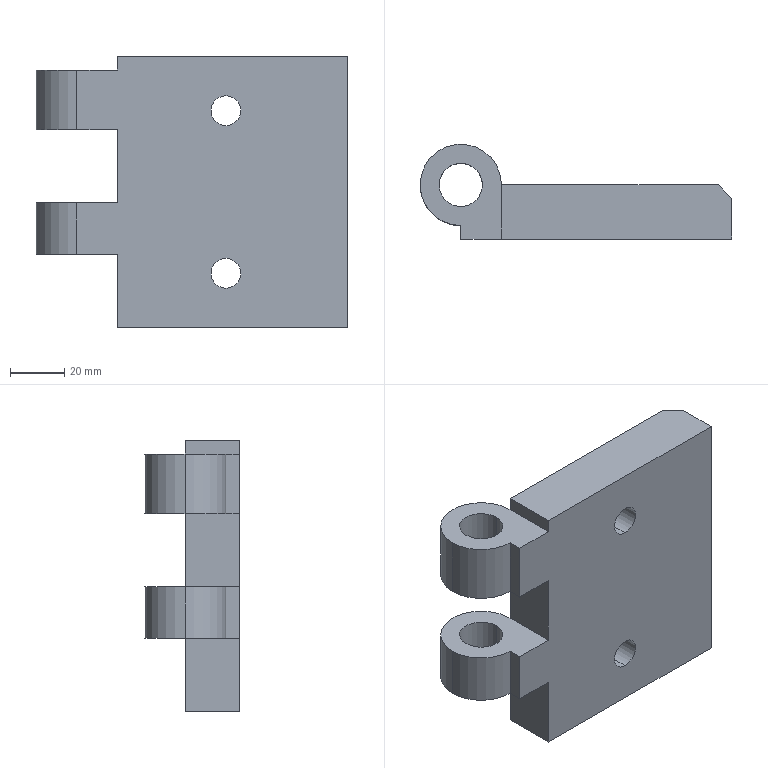Part | SolidWorks | features ICE 2, 3DProfileFeature 1, Chamfer 1, Extrusion 1, HoleWzd 1, MirrorPattern 1 | 1 solid | 33 faces | box 115 x 35 x 100 mm | volume 190454 mm3 | plane 17 | cylinder 16 | commonest cylinder face diameters 11 x4 16 x4 22 x4 30 x4
STEP:
#1=CARTESIAN_POINT('',(5.,9.5,19.));
#2=VERTEX_POINT('',#1);
#3=CARTESIAN_POINT('',(5.,9.5,41.));
#4=VERTEX_POINT('',#3);
#5=CARTESIAN_POINT('',(5.,9.5,30.));
#6=DIRECTION('',(0.,1.,0.));
#7=DIRECTION('',(0.,0.,1.));
#8=AXIS2_PLACEMENT_3D('',#5,#6,#7);
#9=CIRCLE('',#8,11.);
#10=EDGE_CURVE('',#2,#4,#9,.T.);
#11=ORIENTED_EDGE('',*,*,#10,.F.);
#12=CARTESIAN_POINT('',(5.,10.,19.));
#13=VERTEX_POINT('',#12);
#14=CARTESIAN_POINT('',(5.,10.,19.));
#15=DIRECTION('',(0.,1.,0.));
#16=VECTOR('',#15,1000.);
#17=LINE('',#14,#16);
#18=EDGE_CURVE('',#2,#13,#17,.T.);
#19=ORIENTED_EDGE('',*,*,#18,.T.);
#20=CARTESIAN_POINT('',(5.,10.,41.));
#21=VERTEX_POINT('',#20);
#22=CARTESIAN_POINT('',(5.,10.,30.));
#23=DIRECTION('',(0.,1.,0.));
#24=DIRECTION('',(0.,0.,1.));
#25=AXIS2_PLACEMENT_3D('',#22,#23,#24);
#26=CIRCLE('',#25,11.);
#27=EDGE_CURVE('',#13,#21,#26,.T.);
#28=ORIENTED_EDGE('',*,*,#27,.T.);
#29=CARTESIAN_POINT('',(5.,10.,41.));
#30=DIRECTION('',(0.,1.,0.));
#31=VECTOR('',#30,1000.);
#32=LINE('',#29,#31);
#33=EDGE_CURVE('',#4,#21,#32,.T.);
#34=ORIENTED_EDGE('',*,*,#33,.F.);
#35=EDGE_LOOP('',(#11,#19,#28,#34));
#36=FACE_OUTER_BOUND('',#35,.T.);
#37=CARTESIAN_POINT('',(5.,10.,30.));
#38=DIRECTION('',(0.,1.,0.));
#39=DIRECTION('',(0.,0.,1.));
#40=AXIS2_PLACEMENT_3D('',#37,#38,#39);
#41=CYLINDRICAL_SURFACE('',#40,11.);
#42=ADVANCED_FACE('',(#36),#41,.F.);
#43=CARTESIAN_POINT('',(5.,-10.,24.5));
#44=VERTEX_POINT('',#43);
#45=CARTESIAN_POINT('',(5.,-10.,35.5));
#46=VERTEX_POINT('',#45);
#47=CARTESIAN_POINT('',(5.,-10.,30.));
#48=DIRECTION('',(0.,1.,0.));
#49=DIRECTION('',(0.,0.,1.));
#50=AXIS2_PLACEMENT_3D('',#47,#48,#49);
#51=CIRCLE('',#50,5.5);
#52=EDGE_CURVE('',#44,#46,#51,.T.);
#53=ORIENTED_EDGE('',*,*,#52,.F.);
#54=CARTESIAN_POINT('',(5.,9.5,24.5));
#55=VERTEX_POINT('',#54);
#56=CARTESIAN_POINT('',(5.,10.,24.5));
#57=DIRECTION('',(0.,1.,0.));
#58=VECTOR('',#57,1000.);
#59=LINE('',#56,#58);
#60=EDGE_CURVE('',#44,#55,#59,.T.);
#61=ORIENTED_EDGE('',*,*,#60,.T.);
#62=CARTESIAN_POINT('',(5.,9.5,35.5));
#63=VERTEX_POINT('',#62);
#64=CARTESIAN_POINT('',(5.,9.5,30.));
#65=DIRECTION('',(0.,1.,0.));
#66=DIRECTION('',(0.,0.,1.));
#67=AXIS2_PLACEMENT_3D('',#64,#65,#66);
#68=CIRCLE('',#67,5.5);
#69=EDGE_CURVE('',#55,#63,#68,.T.);
#70=ORIENTED_EDGE('',*,*,#69,.T.);
#71=CARTESIAN_POINT('',(5.,10.,35.5));
#72=DIRECTION('',(0.,1.,0.));
#73=VECTOR('',#72,1000.);
#74=LINE('',#71,#73);
#75=EDGE_CURVE('',#46,#63,#74,.T.);
#76=ORIENTED_EDGE('',*,*,#75,.F.);
#77=EDGE_LOOP('',(#53,#61,#70,#76));
#78=FACE_OUTER_BOUND('',#77,.T.);
#79=CARTESIAN_POINT('',(5.,10.,30.));
#80=DIRECTION('',(0.,1.,0.));
#81=DIRECTION('',(0.,0.,1.));
#82=AXIS2_PLACEMENT_3D('',#79,#80,#81);
#83=CYLINDRICAL_SURFACE('',#82,5.5);
#84=ADVANCED_FACE('',(#78),#83,.F.);
#85=CARTESIAN_POINT('',(5.,9.5,-41.));
#86=VERTEX_POINT('',#85);
#87=CARTESIAN_POINT('',(5.,9.5,-19.));
#88=VERTEX_POINT('',#87);
#89=CARTESIAN_POINT('',(5.,9.5,-30.));
#90=DIRECTION('',(0.,1.,0.));
#91=DIRECTION('',(0.,0.,1.));
#92=AXIS2_PLACEMENT_3D('',#89,#90,#91);
#93=CIRCLE('',#92,11.);
#94=EDGE_CURVE('',#86,#88,#93,.T.);
#95=ORIENTED_EDGE('',*,*,#94,.F.);
#96=CARTESIAN_POINT('',(5.,10.,-41.));
#97=VERTEX_POINT('',#96);
#98=CARTESIAN_POINT('',(5.,10.,-41.));
#99=DIRECTION('',(0.,1.,0.));
#100=VECTOR('',#99,1000.);
#101=LINE('',#98,#100);
#102=EDGE_CURVE('',#86,#97,#101,.T.);
#103=ORIENTED_EDGE('',*,*,#102,.T.);
#104=CARTESIAN_POINT('',(5.,10.,-19.));
#105=VERTEX_POINT('',#104);
#106=CARTESIAN_POINT('',(5.,10.,-30.));
#107=DIRECTION('',(0.,1.,0.));
#108=DIRECTION('',(0.,0.,1.));
#109=AXIS2_PLACEMENT_3D('',#106,#107,#108);
#110=CIRCLE('',#109,11.);
#111=EDGE_CURVE('',#97,#105,#110,.T.);
#112=ORIENTED_EDGE('',*,*,#111,.T.);
#113=CARTESIAN_POINT('',(5.,10.,-19.));
#114=DIRECTION('',(0.,1.,0.));
#115=VECTOR('',#114,1000.);
#116=LINE('',#113,#115);
#117=EDGE_CURVE('',#88,#105,#116,.T.);
#118=ORIENTED_EDGE('',*,*,#117,.F.);
#119=EDGE_LOOP('',(#95,#103,#112,#118));
#120=FACE_OUTER_BOUND('',#119,.T.);
#121=CARTESIAN_POINT('',(5.,10.,-30.));
#122=DIRECTION('',(0.,1.,0.));
#123=DIRECTION('',(0.,0.,1.));
#124=AXIS2_PLACEMENT_3D('',#121,#122,#123);
#125=CYLINDRICAL_SURFACE('',#124,11.);
#126=ADVANCED_FACE('',(#120),#125,.F.);
#127=CARTESIAN_POINT('',(5.,-10.,-35.5));
#128=VERTEX_POINT('',#127);
#129=CARTESIAN_POINT('',(5.,-10.,-24.5));
#130=VERTEX_POINT('',#129);
#131=CARTESIAN_POINT('',(5.,-10.,-30.));
#132=DIRECTION('',(0.,1.,0.));
#133=DIRECTION('',(0.,0.,1.));
#134=AXIS2_PLACEMENT_3D('',#131,#132,#133);
#135=CIRCLE('',#134,5.5);
#136=EDGE_CURVE('',#128,#130,#135,.T.);
#137=ORIENTED_EDGE('',*,*,#136,.F.);
#138=CARTESIAN_POINT('',(5.,9.5,-35.5));
#139=VERTEX_POINT('',#138);
#140=CARTESIAN_POINT('',(5.,10.,-35.5));
#141=DIRECTION('',(0.,1.,0.));
#142=VECTOR('',#141,1000.);
#143=LINE('',#140,#142);
#144=EDGE_CURVE('',#128,#139,#143,.T.);
#145=ORIENTED_EDGE('',*,*,#144,.T.);
#146=CARTESIAN_POINT('',(5.,9.5,-24.5));
#147=VERTEX_POINT('',#146);
#148=CARTESIAN_POINT('',(5.,9.5,-30.));
#149=DIRECTION('',(0.,1.,0.));
#150=DIRECTION('',(0.,0.,1.));
#151=AXIS2_PLACEMENT_3D('',#148,#149,#150);
#152=CIRCLE('',#151,5.5);
#153=EDGE_CURVE('',#139,#147,#152,.T.);
#154=ORIENTED_EDGE('',*,*,#153,.T.);
#155=CARTESIAN_POINT('',(5.,10.,-24.5));
#156=DIRECTION('',(0.,1.,0.));
#157=VECTOR('',#156,1000.);
#158=LINE('',#155,#157);
#159=EDGE_CURVE('',#130,#147,#158,.T.);
#160=ORIENTED_EDGE('',*,*,#159,.F.);
#161=EDGE_LOOP('',(#137,#145,#154,#160));
#162=FACE_OUTER_BOUND('',#161,.T.);
#163=CARTESIAN_POINT('',(5.,10.,-30.));
#164=DIRECTION('',(0.,1.,0.));
#165=DIRECTION('',(0.,0.,1.));
#166=AXIS2_PLACEMENT_3D('',#163,#164,#165);
#167=CYLINDRICAL_SURFACE('',#166,5.5);
#168=ADVANCED_FACE('',(#162),#167,.F.);
#169=CARTESIAN_POINT('',(-42.,10.,-22.997));
#170=VERTEX_POINT('',#169);
#171=CARTESIAN_POINT('',(-58.,10.,-22.997));
#172=VERTEX_POINT('',#171);
#173=CARTESIAN_POINT('',(-50.,10.,-22.997));
#174=DIRECTION('',(0.,0.,-1.));
#175=DIRECTION('',(1.,0.,0.));
#176=AXIS2_PLACEMENT_3D('',#173,#174,#175);
#177=CIRCLE('',#176,8.);
#178=EDGE_CURVE('',#170,#172,#177,.T.);
#179=ORIENTED_EDGE('',*,*,#178,.T.);
#180=CARTESIAN_POINT('',(-58.,10.,-3.997));
#181=VERTEX_POINT('',#180);
#182=CARTESIAN_POINT('',(-58.,10.,-50.));
#183=DIRECTION('',(0.,0.,1.));
#184=VECTOR('',#183,1000.);
#185=LINE('',#182,#184);
#186=EDGE_CURVE('',#172,#181,#185,.T.);
#187=ORIENTED_EDGE('',*,*,#186,.T.);
#188=CARTESIAN_POINT('',(-42.,10.,-3.997));
#189=VERTEX_POINT('',#188);
#190=CARTESIAN_POINT('',(-50.,10.,-3.997));
#191=DIRECTION('',(0.,0.,-1.));
#192=DIRECTION('',(1.,0.,0.));
#193=AXIS2_PLACEMENT_3D('',#190,#191,#192);
#194=CIRCLE('',#193,8.);
#195=EDGE_CURVE('',#189,#181,#194,.T.);
#196=ORIENTED_EDGE('',*,*,#195,.F.);
#197=CARTESIAN_POINT('',(-42.,10.,-50.));
#198=DIRECTION('',(0.,0.,1.));
#199=VECTOR('',#198,1000.);
#200=LINE('',#197,#199);
#201=EDGE_CURVE('',#170,#189,#200,.T.);
#202=ORIENTED_EDGE('',*,*,#201,.F.);
#203=EDGE_LOOP('',(#179,#187,#196,#202));
#204=FACE_OUTER_BOUND('',#203,.T.);
#205=CARTESIAN_POINT('',(-50.,10.,-50.));
#206=DIRECTION('',(0.,0.,1.));
#207=DIRECTION('',(1.,0.,0.));
#208=AXIS2_PLACEMENT_3D('',#205,#206,#207);
#209=CYLINDRICAL_SURFACE('',#208,8.);
#210=ADVANCED_FACE('',(#204),#209,.F.);
#211=CARTESIAN_POINT('',(-42.,10.,23.003));
#212=VERTEX_POINT('',#211);
#213=CARTESIAN_POINT('',(-58.,10.,23.003));
#214=VERTEX_POINT('',#213);
#215=CARTESIAN_POINT('',(-50.,10.,23.003));
#216=DIRECTION('',(0.,0.,-1.));
#217=DIRECTION('',(1.,0.,0.));
#218=AXIS2_PLACEMENT_3D('',#215,#216,#217);
#219=CIRCLE('',#218,8.);
#220=EDGE_CURVE('',#212,#214,#219,.T.);
#221=ORIENTED_EDGE('',*,*,#220,.T.);
#222=CARTESIAN_POINT('',(-58.,10.,45.));
#223=VERTEX_POINT('',#222);
#224=CARTESIAN_POINT('',(-58.,10.,-50.));
#225=DIRECTION('',(0.,0.,1.));
#226=VECTOR('',#225,1000.);
#227=LINE('',#224,#226);
#228=EDGE_CURVE('',#214,#223,#227,.T.);
#229=ORIENTED_EDGE('',*,*,#228,.T.);
#230=CARTESIAN_POINT('',(-42.,10.,45.));
#231=VERTEX_POINT('',#230);
#232=CARTESIAN_POINT('',(-50.,10.,45.));
#233=DIRECTION('',(0.,0.,1.));
#234=DIRECTION('',(-1.,0.,0.));
#235=AXIS2_PLACEMENT_3D('',#232,#233,#234);
#236=CIRCLE('',#235,8.);
#237=EDGE_CURVE('',#223,#231,#236,.T.);
#238=ORIENTED_EDGE('',*,*,#237,.T.);
#239=CARTESIAN_POINT('',(-42.,10.,-50.));
#240=DIRECTION('',(0.,0.,1.));
#241=VECTOR('',#240,1000.);
#242=LINE('',#239,#241);
#243=EDGE_CURVE('',#212,#231,#242,.T.);
#244=ORIENTED_EDGE('',*,*,#243,.F.);
#245=EDGE_LOOP('',(#221,#229,#238,#244));
#246=FACE_OUTER_BOUND('',#245,.T.);
#247=CARTESIAN_POINT('',(-50.,10.,-50.));
#248=DIRECTION('',(0.,0.,1.));
#249=DIRECTION('',(1.,0.,0.));
#250=AXIS2_PLACEMENT_3D('',#247,#248,#249);
#251=CYLINDRICAL_SURFACE('',#250,8.);
#252=ADVANCED_FACE('',(#246),#251,.F.);
#253=CARTESIAN_POINT('',(-50.,-5.,45.));
#254=VERTEX_POINT('',#253);
#255=CARTESIAN_POINT('',(-65.,10.,45.));
#256=VERTEX_POINT('',#255);
#257=CARTESIAN_POINT('',(-50.,10.,45.));
#258=DIRECTION('',(0.,0.,-1.));
#259=DIRECTION('',(-1.,0.,0.));
#260=AXIS2_PLACEMENT_3D('',#257,#258,#259);
#261=CIRCLE('',#260,15.);
#262=EDGE_CURVE('',#254,#256,#261,.T.);
#263=ORIENTED_EDGE('',*,*,#262,.T.);
#264=CARTESIAN_POINT('',(-65.,10.,23.003));
#265=VERTEX_POINT('',#264);
#266=CARTESIAN_POINT('',(-65.,10.,50.));
#267=DIRECTION('',(0.,0.,-1.));
#268=VECTOR('',#267,1000.);
#269=LINE('',#266,#268);
#270=EDGE_CURVE('',#256,#265,#269,.T.);
#271=ORIENTED_EDGE('',*,*,#270,.T.);
#272=CARTESIAN_POINT('',(-50.,-5.,23.003));
#273=VERTEX_POINT('',#272);
#274=CARTESIAN_POINT('',(-50.,10.,23.003));
#275=DIRECTION('',(0.,0.,1.));
#276=DIRECTION('',(1.,0.,0.));
#277=AXIS2_PLACEMENT_3D('',#274,#275,#276);
#278=CIRCLE('',#277,15.);
#279=EDGE_CURVE('',#265,#273,#278,.T.);
#280=ORIENTED_EDGE('',*,*,#279,.T.);
#281=CARTESIAN_POINT('',(-50.,-5.,50.));
#282=DIRECTION('',(0.,0.,-1.));
#283=VECTOR('',#282,1000.);
#284=LINE('',#281,#283);
#285=EDGE_CURVE('',#254,#273,#284,.T.);
#286=ORIENTED_EDGE('',*,*,#285,.F.);
#287=EDGE_LOOP('',(#263,#271,#280,#286));
#288=FACE_OUTER_BOUND('',#287,.T.);
#289=CARTESIAN_POINT('',(-50.,10.,50.));
#290=DIRECTION('',(0.,0.,-1.));
#291=DIRECTION('',(-1.,0.,0.));
#292=AXIS2_PLACEMENT_3D('',#289,#290,#291);
#293=CYLINDRICAL_SURFACE('',#292,15.);
#294=ADVANCED_FACE('',(#288),#293,.T.);
#295=CARTESIAN_POINT('',(-65.,10.,-3.997));
#296=VERTEX_POINT('',#295);
#297=CARTESIAN_POINT('',(-50.,-5.,-3.997));
#298=VERTEX_POINT('',#297);
#299=CARTESIAN_POINT('',(-50.,10.,-3.997));
#300=DIRECTION('',(0.,0.,1.));
#301=DIRECTION('',(1.,0.,0.));
#302=AXIS2_PLACEMENT_3D('',#299,#300,#301);
#303=CIRCLE('',#302,15.);
#304=EDGE_CURVE('',#296,#298,#303,.T.);
#305=ORIENTED_EDGE('',*,*,#304,.F.);
#306=CARTESIAN_POINT('',(-65.,10.,-22.997));
#307=VERTEX_POINT('',#306);
#308=CARTESIAN_POINT('',(-65.,10.,50.));
#309=DIRECTION('',(0.,0.,-1.));
#310=VECTOR('',#309,1000.);
#311=LINE('',#308,#310);
#312=EDGE_CURVE('',#296,#307,#311,.T.);
#313=ORIENTED_EDGE('',*,*,#312,.T.);
#314=CARTESIAN_POINT('',(-50.,-5.,-22.997));
#315=VERTEX_POINT('',#314);
#316=CARTESIAN_POINT('',(-50.,10.,-22.997));
#317=DIRECTION('',(0.,0.,1.));
#318=DIRECTION('',(1.,0.,0.));
#319=AXIS2_PLACEMENT_3D('',#316,#317,#318);
#320=CIRCLE('',#319,15.);
#321=EDGE_CURVE('',#307,#315,#320,.T.);
#322=ORIENTED_EDGE('',*,*,#321,.T.);
#323=CARTESIAN_POINT('',(-50.,-5.,50.));
#324=DIRECTION('',(0.,0.,-1.));
#325=VECTOR('',#324,1000.);
#326=LINE('',#323,#325);
#327=EDGE_CURVE('',#298,#315,#326,.T.);
#328=ORIENTED_EDGE('',*,*,#327,.F.);
#329=EDGE_LOOP('',(#305,#313,#322,#328));
#330=FACE_OUTER_BOUND('',#329,.T.);
#331=CARTESIAN_POINT('',(-50.,10.,50.));
#332=DIRECTION('',(0.,0.,-1.));
#333=DIRECTION('',(-1.,0.,0.));
#334=AXIS2_PLACEMENT_3D('',#331,#332,#333);
#335=CYLINDRICAL_SURFACE('',#334,15.);
#336=ADVANCED_FACE('',(#330),#335,.T.);
#337=CARTESIAN_POINT('',(5.,10.,30.));
#338=DIRECTION('',(0.,1.,0.));
#339=DIRECTION('',(0.,0.,1.));
#340=AXIS2_PLACEMENT_3D('',#337,#338,#339);
#341=CIRCLE('',#340,11.);
#342=EDGE_CURVE('',#21,#13,#341,.T.);
#343=ORIENTED_EDGE('',*,*,#342,.F.);
#344=ORIENTED_EDGE('',*,*,#27,.F.);
#345=EDGE_LOOP('',(#343,#344));
#346=FACE_BOUND('',#345,.T.);
#347=CARTESIAN_POINT('',(45.,10.,50.));
#348=VERTEX_POINT('',#347);
#349=CARTESIAN_POINT('',(-35.,10.,50.));
#350=VERTEX_POINT('',#349);
#351=CARTESIAN_POINT('',(-35.,10.,50.));
#352=DIRECTION('',(-1.,0.,0.));
#353=VECTOR('',#352,1000.);
#354=LINE('',#351,#353);
#355=EDGE_CURVE('',#348,#350,#354,.T.);
#356=ORIENTED_EDGE('',*,*,#355,.F.);
#357=CARTESIAN_POINT('',(45.,10.,-50.));
#358=VERTEX_POINT('',#357);
#359=CARTESIAN_POINT('',(45.,10.,50.));
#360=DIRECTION('',(0.,0.,-1.));
#361=VECTOR('',#360,1000.);
#362=LINE('',#359,#361);
#363=EDGE_CURVE('',#348,#358,#362,.T.);
#364=ORIENTED_EDGE('',*,*,#363,.T.);
#365=CARTESIAN_POINT('',(-35.,10.,-50.));
#366=VERTEX_POINT('',#365);
#367=CARTESIAN_POINT('',(-35.,10.,-50.));
#368=DIRECTION('',(-1.,0.,0.));
#369=VECTOR('',#368,1000.);
#370=LINE('',#367,#369);
#371=EDGE_CURVE('',#358,#366,#370,.T.);
#372=ORIENTED_EDGE('',*,*,#371,.T.);
#373=CARTESIAN_POINT('',(-35.,10.,-22.997));
#374=VERTEX_POINT('',#373);
#375=CARTESIAN_POINT('',(-35.,10.,50.));
#376=DIRECTION('',(0.,0.,-1.));
#377=VECTOR('',#376,1000.);
#378=LINE('',#375,#377);
#379=EDGE_CURVE('',#374,#366,#378,.T.);
#380=ORIENTED_EDGE('',*,*,#379,.F.);
#381=CARTESIAN_POINT('',(-35.,10.,-3.997));
#382=VERTEX_POINT('',#381);
#383=CARTESIAN_POINT('',(-35.,10.,50.));
#384=DIRECTION('',(0.,0.,-1.));
#385=VECTOR('',#384,1000.);
#386=LINE('',#383,#385);
#387=EDGE_CURVE('',#382,#374,#386,.T.);
#388=ORIENTED_EDGE('',*,*,#387,.F.);
#389=CARTESIAN_POINT('',(-35.,10.,23.003));
#390=VERTEX_POINT('',#389);
#391=CARTESIAN_POINT('',(-35.,10.,50.));
#392=DIRECTION('',(0.,0.,-1.));
#393=VECTOR('',#392,1000.);
#394=LINE('',#391,#393);
#395=EDGE_CURVE('',#390,#382,#394,.T.);
#396=ORIENTED_EDGE('',*,*,#395,.F.);
#397=CARTESIAN_POINT('',(-35.,10.,45.));
#398=VERTEX_POINT('',#397);
#399=CARTESIAN_POINT('',(-35.,10.,50.));
#400=DIRECTION('',(0.,0.,-1.));
#401=VECTOR('',#400,1000.);
#402=LINE('',#399,#401);
#403=EDGE_CURVE('',#398,#390,#402,.T.);
#404=ORIENTED_EDGE('',*,*,#403,.F.);
#405=CARTESIAN_POINT('',(-35.,10.,50.));
#406=DIRECTION('',(0.,0.,-1.));
#407=VECTOR('',#406,1000.);
#408=LINE('',#405,#407);
#409=EDGE_CURVE('',#350,#398,#408,.T.);
#410=ORIENTED_EDGE('',*,*,#409,.F.);
#411=EDGE_LOOP('',(#356,#364,#372,#380,#388,#396,#404,#410));
#412=FACE_OUTER_BOUND('',#411,.T.);
#413=CARTESIAN_POINT('',(5.,10.,-30.));
#414=DIRECTION('',(0.,1.,0.));
#415=DIRECTION('',(0.,0.,1.));
#416=AXIS2_PLACEMENT_3D('',#413,#414,#415);
#417=CIRCLE('',#416,11.);
#418=EDGE_CURVE('',#105,#97,#417,.T.);
#419=ORIENTED_EDGE('',*,*,#418,.F.);
#420=ORIENTED_EDGE('',*,*,#111,.F.);
#421=EDGE_LOOP('',(#419,#420));
#422=FACE_BOUND('',#421,.T.);
#423=CARTESIAN_POINT('',(-35.,10.,50.));
#424=DIRECTION('',(0.,-1.,0.));
#425=DIRECTION('',(0.,0.,-1.));
#426=AXIS2_PLACEMENT_3D('',#423,#424,#425);
#427=PLANE('',#426);
#428=ADVANCED_FACE('',(#346,#412,#422),#427,.F.);
#429=ORIENTED_EDGE('',*,*,#312,.F.);
#430=CARTESIAN_POINT('',(-50.,10.,-3.997));
#431=DIRECTION('',(0.,0.,1.));
#432=DIRECTION('',(1.,0.,0.));
#433=AXIS2_PLACEMENT_3D('',#430,#431,#432);
#434=CIRCLE('',#433,15.);
#435=EDGE_CURVE('',#382,#296,#434,.T.);
#436=ORIENTED_EDGE('',*,*,#435,.F.);
#437=ORIENTED_EDGE('',*,*,#387,.T.);
#438=CARTESIAN_POINT('',(-50.,10.,-22.997));
#439=DIRECTION('',(0.,0.,1.));
#440=DIRECTION('',(1.,0.,0.));
#441=AXIS2_PLACEMENT_3D('',#438,#439,#440);
#442=CIRCLE('',#441,15.);
#443=EDGE_CURVE('',#374,#307,#442,.T.);
#444=ORIENTED_EDGE('',*,*,#443,.T.);
#445=EDGE_LOOP('',(#429,#436,#437,#444));
#446=FACE_OUTER_BOUND('',#445,.T.);
#447=CARTESIAN_POINT('',(-50.,10.,50.));
#448=DIRECTION('',(0.,0.,-1.));
#449=DIRECTION('',(-1.,0.,0.));
#450=AXIS2_PLACEMENT_3D('',#447,#448,#449);
#451=CYLINDRICAL_SURFACE('',#450,15.);
#452=ADVANCED_FACE('',(#446),#451,.T.);
#453=ORIENTED_EDGE('',*,*,#327,.T.);
#454=CARTESIAN_POINT('',(-50.,-10.,-22.997));
#455=VERTEX_POINT('',#454);
#456=CARTESIAN_POINT('',(-50.,-10.,-22.997));
#457=DIRECTION('',(0.,-1.,0.));
#458=VECTOR('',#457,1000.);
#459=LINE('',#456,#458);
#460=EDGE_CURVE('',#315,#455,#459,.T.);
#461=ORIENTED_EDGE('',*,*,#460,.T.);
#462=CARTESIAN_POINT('',(-50.,-10.,-3.997));
#463=VERTEX_POINT('',#462);
#464=CARTESIAN_POINT('',(-50.,-10.,50.));
#465=DIRECTION('',(0.,0.,-1.));
#466=VECTOR('',#465,1000.);
#467=LINE('',#464,#466);
#468=EDGE_CURVE('',#463,#455,#467,.T.);
#469=ORIENTED_EDGE('',*,*,#468,.F.);
#470=CARTESIAN_POINT('',(-50.,-10.,-3.997));
#471=DIRECTION('',(0.,-1.,0.));
#472=VECTOR('',#471,1000.);
#473=LINE('',#470,#472);
#474=EDGE_CURVE('',#298,#463,#473,.T.);
#475=ORIENTED_EDGE('',*,*,#474,.F.);
#476=EDGE_LOOP('',(#453,#461,#469,#475));
#477=FACE_OUTER_BOUND('',#476,.T.);
#478=CARTESIAN_POINT('',(-50.,-10.,50.));
#479=DIRECTION('',(1.,0.,0.));
#480=DIRECTION('',(0.,0.,-1.));
#481=AXIS2_PLACEMENT_3D('',#478,#479,#480);
#482=PLANE('',#481);
#483=ADVANCED_FACE('',(#477),#482,.F.);
#484=CARTESIAN_POINT('',(5.,-10.,30.));
#485=DIRECTION('',(0.,1.,0.));
#486=DIRECTION('',(0.,0.,1.));
#487=AXIS2_PLACEMENT_3D('',#484,#485,#486);
#488=CIRCLE('',#487,5.5);
#489=EDGE_CURVE('',#46,#44,#488,.T.);
#490=ORIENTED_EDGE('',*,*,#489,.T.);
#491=ORIENTED_EDGE('',*,*,#52,.T.);
#492=EDGE_LOOP('',(#490,#491));
#493=FACE_BOUND('',#492,.T.);
#494=CARTESIAN_POINT('',(5.,-10.,-30.));
#495=DIRECTION('',(0.,1.,0.));
#496=DIRECTION('',(0.,0.,1.));
#497=AXIS2_PLACEMENT_3D('',#494,#495,#496);
#498=CIRCLE('',#497,5.5);
#499=EDGE_CURVE('',#130,#128,#498,.T.);
#500=ORIENTED_EDGE('',*,*,#499,.T.);
#501=ORIENTED_EDGE('',*,*,#136,.T.);
#502=EDGE_LOOP('',(#500,#501));
#503=FACE_BOUND('',#502,.T.);
#504=CARTESIAN_POINT('',(-35.,-10.,-50.));
#505=VERTEX_POINT('',#504);
#506=CARTESIAN_POINT('',(-35.,-10.,-22.997));
#507=VERTEX_POINT('',#506);
#508=CARTESIAN_POINT('',(-35.,-10.,0.));
#509=DIRECTION('',(0.,0.,1.));
#510=VECTOR('',#509,1000.);
#511=LINE('',#508,#510);
#512=EDGE_CURVE('',#505,#507,#511,.T.);
#513=ORIENTED_EDGE('',*,*,#512,.F.);
#514=CARTESIAN_POINT('',(50.,-10.,-50.));
#515=VERTEX_POINT('',#514);
#516=CARTESIAN_POINT('',(-50.,-10.,-50.));
#517=DIRECTION('',(1.,0.,0.));
#518=VECTOR('',#517,1000.);
#519=LINE('',#516,#518);
#520=EDGE_CURVE('',#505,#515,#519,.T.);
#521=ORIENTED_EDGE('',*,*,#520,.T.);
#522=CARTESIAN_POINT('',(50.,-10.,50.));
#523=VERTEX_POINT('',#522);
#524=CARTESIAN_POINT('',(50.,-10.,50.));
#525=DIRECTION('',(0.,0.,-1.));
#526=VECTOR('',#525,1000.);
#527=LINE('',#524,#526);
#528=EDGE_CURVE('',#523,#515,#527,.T.);
#529=ORIENTED_EDGE('',*,*,#528,.F.);
#530=CARTESIAN_POINT('',(-35.,-10.,50.));
#531=VERTEX_POINT('',#530);
#532=CARTESIAN_POINT('',(-50.,-10.,50.));
#533=DIRECTION('',(1.,0.,0.));
#534=VECTOR('',#533,1000.);
#535=LINE('',#532,#534);
#536=EDGE_CURVE('',#531,#523,#535,.T.);
#537=ORIENTED_EDGE('',*,*,#536,.F.);
#538=CARTESIAN_POINT('',(-35.,-10.,45.));
#539=VERTEX_POINT('',#538);
#540=CARTESIAN_POINT('',(-35.,-10.,50.));
#541=DIRECTION('',(0.,0.,-1.));
#542=VECTOR('',#541,1000.);
#543=LINE('',#540,#542);
#544=EDGE_CURVE('',#531,#539,#543,.T.);
#545=ORIENTED_EDGE('',*,*,#544,.T.);
#546=CARTESIAN_POINT('',(-50.,-10.,45.));
#547=VERTEX_POINT('',#546);
#548=CARTESIAN_POINT('',(-35.,-10.,45.));
#549=DIRECTION('',(-1.,0.,0.));
#550=VECTOR('',#549,1000.);
#551=LINE('',#548,#550);
#552=EDGE_CURVE('',#539,#547,#551,.T.);
#553=ORIENTED_EDGE('',*,*,#552,.T.);
#554=CARTESIAN_POINT('',(-50.,-10.,23.003));
#555=VERTEX_POINT('',#554);
#556=CARTESIAN_POINT('',(-50.,-10.,50.));
#557=DIRECTION('',(0.,0.,-1.));
#558=VECTOR('',#557,1000.);
#559=LINE('',#556,#558);
#560=EDGE_CURVE('',#547,#555,#559,.T.);
#561=ORIENTED_EDGE('',*,*,#560,.T.);
#562=CARTESIAN_POINT('',(-35.,-10.,23.003));
#563=VERTEX_POINT('',#562);
#564=CARTESIAN_POINT('',(-69.568,-10.,23.003));
#565=DIRECTION('',(1.,0.,0.));
#566=VECTOR('',#565,1000.);
#567=LINE('',#564,#566);
#568=EDGE_CURVE('',#555,#563,#567,.T.);
#569=ORIENTED_EDGE('',*,*,#568,.T.);
#570=CARTESIAN_POINT('',(-35.,-10.,-3.997));
#571=VERTEX_POINT('',#570);
#572=CARTESIAN_POINT('',(-35.,-10.,23.003));
#573=DIRECTION('',(0.,0.,-1.));
#574=VECTOR('',#573,1000.);
#575=LINE('',#572,#574);
#576=EDGE_CURVE('',#563,#571,#575,.T.);
#577=ORIENTED_EDGE('',*,*,#576,.T.);
#578=CARTESIAN_POINT('',(-69.568,-10.,-3.997));
#579=DIRECTION('',(1.,0.,0.));
#580=VECTOR('',#579,1000.);
#581=LINE('',#578,#580);
#582=EDGE_CURVE('',#463,#571,#581,.T.);
#583=ORIENTED_EDGE('',*,*,#582,.F.);
#584=ORIENTED_EDGE('',*,*,#468,.T.);
#585=CARTESIAN_POINT('',(0.,-10.,-22.997));
#586=DIRECTION('',(1.,0.,0.));
#587=VECTOR('',#586,1000.);
#588=LINE('',#585,#587);
#589=EDGE_CURVE('',#455,#507,#588,.T.);
#590=ORIENTED_EDGE('',*,*,#589,.T.);
#591=EDGE_LOOP('',(#513,#521,#529,#537,#545,#553,#561,#569,#577,#583,#584,#590));
#592=FACE_OUTER_BOUND('',#591,.T.);
#593=CARTESIAN_POINT('',(-50.,-10.,50.));
#594=DIRECTION('',(0.,1.,0.));
#595=DIRECTION('',(0.,0.,1.));
#596=AXIS2_PLACEMENT_3D('',#593,#594,#595);
#597=PLANE('',#596);
#598=ADVANCED_FACE('',(#493,#503,#592),#597,.F.);
#599=ORIENTED_EDGE('',*,*,#371,.F.);
#600=CARTESIAN_POINT('',(50.,5.,-50.));
#601=VERTEX_POINT('',#600);
#602=CARTESIAN_POINT('',(45.,10.,-50.));
#603=DIRECTION('',(0.7071,-0.7071,0.));
#604=VECTOR('',#603,1000.);
#605=LINE('',#602,#604);
#606=EDGE_CURVE('',#358,#601,#605,.T.);
#607=ORIENTED_EDGE('',*,*,#606,.T.);
#608=CARTESIAN_POINT('',(50.,-10.,-50.));
#609=DIRECTION('',(0.,1.,0.));
#610=VECTOR('',#609,1000.);
#611=LINE('',#608,#610);
#612=EDGE_CURVE('',#515,#601,#611,.T.);
#613=ORIENTED_EDGE('',*,*,#612,.F.);
#614=ORIENTED_EDGE('',*,*,#520,.F.);
#615=CARTESIAN_POINT('',(-35.,-10.,-50.));
#616=DIRECTION('',(0.,1.,0.));
#617=VECTOR('',#616,1000.);
#618=LINE('',#615,#617);
#619=EDGE_CURVE('',#505,#366,#618,.T.);
#620=ORIENTED_EDGE('',*,*,#619,.T.);
#621=EDGE_LOOP('',(#599,#607,#613,#614,#620));
#622=FACE_OUTER_BOUND('',#621,.T.);
#623=CARTESIAN_POINT('',(-50.,10.,-50.));
#624=DIRECTION('',(0.,0.,1.));
#625=DIRECTION('',(1.,0.,0.));
#626=AXIS2_PLACEMENT_3D('',#623,#624,#625);
#627=PLANE('',#626);
#628=ADVANCED_FACE('',(#622),#627,.F.);
#629=ORIENTED_EDGE('',*,*,#612,.T.);
#630=CARTESIAN_POINT('',(50.,5.,50.));
#631=VERTEX_POINT('',#630);
#632=CARTESIAN_POINT('',(50.,5.,50.));
#633=DIRECTION('',(0.,0.,1.));
#634=VECTOR('',#633,1000.);
#635=LINE('',#632,#634);
#636=EDGE_CURVE('',#601,#631,#635,.T.);
#637=ORIENTED_EDGE('',*,*,#636,.T.);
#638=CARTESIAN_POINT('',(50.,-10.,50.));
#639=DIRECTION('',(0.,1.,0.));
#640=VECTOR('',#639,1000.);
#641=LINE('',#638,#640);
#642=EDGE_CURVE('',#523,#631,#641,.T.);
#643=ORIENTED_EDGE('',*,*,#642,.F.);
#644=ORIENTED_EDGE('',*,*,#528,.T.);
#645=EDGE_LOOP('',(#629,#637,#643,#644));
#646=FACE_OUTER_BOUND('',#645,.T.);
#647=CARTESIAN_POINT('',(50.,-10.,50.));
#648=DIRECTION('',(-1.,0.,0.));
#649=DIRECTION('',(0.,0.,1.));
#650=AXIS2_PLACEMENT_3D('',#647,#648,#649);
#651=PLANE('',#650);
#652=ADVANCED_FACE('',(#646),#651,.F.);
#653=ORIENTED_EDGE('',*,*,#270,.F.);
#654=CARTESIAN_POINT('',(-50.,10.,45.));
#655=DIRECTION('',(0.,0.,-1.));
#656=DIRECTION('',(-1.,0.,0.));
#657=AXIS2_PLACEMENT_3D('',#654,#655,#656);
#658=CIRCLE('',#657,15.);
#659=EDGE_CURVE('',#256,#398,#658,.T.);
#660=ORIENTED_EDGE('',*,*,#659,.T.);
#661=ORIENTED_EDGE('',*,*,#403,.T.);
#662=CARTESIAN_POINT('',(-50.,10.,23.003));
#663=DIRECTION('',(0.,0.,1.));
#664=DIRECTION('',(1.,0.,0.));
#665=AXIS2_PLACEMENT_3D('',#662,#663,#664);
#666=CIRCLE('',#665,15.);
#667=EDGE_CURVE('',#390,#265,#666,.T.);
#668=ORIENTED_EDGE('',*,*,#667,.T.);
#669=EDGE_LOOP('',(#653,#660,#661,#668));
#670=FACE_OUTER_BOUND('',#669,.T.);
#671=CARTESIAN_POINT('',(-50.,10.,50.));
#672=DIRECTION('',(0.,0.,-1.));
#673=DIRECTION('',(-1.,0.,0.));
#674=AXIS2_PLACEMENT_3D('',#671,#672,#673);
#675=CYLINDRICAL_SURFACE('',#674,15.);
#676=ADVANCED_FACE('',(#670),#675,.T.);
#677=ORIENTED_EDGE('',*,*,#285,.T.);
#678=CARTESIAN_POINT('',(-50.,-10.,23.003));
#679=DIRECTION('',(0.,-1.,0.));
#680=VECTOR('',#679,1000.);
#681=LINE('',#678,#680);
#682=EDGE_CURVE('',#273,#555,#681,.T.);
#683=ORIENTED_EDGE('',*,*,#682,.T.);
#684=ORIENTED_EDGE('',*,*,#560,.F.);
#685=CARTESIAN_POINT('',(-50.,-10.,45.));
#686=DIRECTION('',(0.,1.,0.));
#687=VECTOR('',#686,1000.);
#688=LINE('',#685,#687);
#689=EDGE_CURVE('',#547,#254,#688,.T.);
#690=ORIENTED_EDGE('',*,*,#689,.T.);
#691=EDGE_LOOP('',(#677,#683,#684,#690));
#692=FACE_OUTER_BOUND('',#691,.T.);
#693=CARTESIAN_POINT('',(-50.,-10.,50.));
#694=DIRECTION('',(1.,0.,0.));
#695=DIRECTION('',(0.,0.,-1.));
#696=AXIS2_PLACEMENT_3D('',#693,#694,#695);
#697=PLANE('',#696);
#698=ADVANCED_FACE('',(#692),#697,.F.);
#699=ORIENTED_EDGE('',*,*,#642,.T.);
#700=CARTESIAN_POINT('',(-2.5,57.5,50.));
#701=DIRECTION('',(-0.7071,0.7071,0.));
#702=VECTOR('',#701,1000.);
#703=LINE('',#700,#702);
#704=EDGE_CURVE('',#631,#348,#703,.T.);
#705=ORIENTED_EDGE('',*,*,#704,.T.);
#706=ORIENTED_EDGE('',*,*,#355,.T.);
#707=CARTESIAN_POINT('',(-35.,-10.,50.));
#708=DIRECTION('',(0.,1.,0.));
#709=VECTOR('',#708,1000.);
#710=LINE('',#707,#709);
#711=EDGE_CURVE('',#531,#350,#710,.T.);
#712=ORIENTED_EDGE('',*,*,#711,.F.);
#713=ORIENTED_EDGE('',*,*,#536,.T.);
#714=EDGE_LOOP('',(#699,#705,#706,#712,#713));
#715=FACE_OUTER_BOUND('',#714,.T.);
#716=CARTESIAN_POINT('',(-50.,10.,50.));
#717=DIRECTION('',(0.,0.,1.));
#718=DIRECTION('',(1.,0.,0.));
#719=AXIS2_PLACEMENT_3D('',#716,#717,#718);
#720=PLANE('',#719);
#721=ADVANCED_FACE('',(#715),#720,.T.);
#722=CARTESIAN_POINT('',(-50.,10.,45.));
#723=DIRECTION('',(0.,0.,1.));
#724=DIRECTION('',(-1.,0.,0.));
#725=AXIS2_PLACEMENT_3D('',#722,#723,#724);
#726=CIRCLE('',#725,8.);
#727=EDGE_CURVE('',#231,#223,#726,.T.);
#728=ORIENTED_EDGE('',*,*,#727,.F.);
#729=ORIENTED_EDGE('',*,*,#237,.F.);
#730=EDGE_LOOP('',(#728,#729));
#731=FACE_BOUND('',#730,.T.);
#732=ORIENTED_EDGE('',*,*,#262,.F.);
#733=ORIENTED_EDGE('',*,*,#689,.F.);
#734=ORIENTED_EDGE('',*,*,#552,.F.);
#735=CARTESIAN_POINT('',(-35.,-10.,45.));
#736=DIRECTION('',(0.,1.,0.));
#737=VECTOR('',#736,1000.);
#738=LINE('',#735,#737);
#739=EDGE_CURVE('',#539,#398,#738,.T.);
#740=ORIENTED_EDGE('',*,*,#739,.T.);
#741=ORIENTED_EDGE('',*,*,#659,.F.);
#742=EDGE_LOOP('',(#732,#733,#734,#740,#741));
#743=FACE_OUTER_BOUND('',#742,.T.);
#744=CARTESIAN_POINT('',(-35.,-10.,45.));
#745=DIRECTION('',(0.,0.,-1.));
#746=DIRECTION('',(-1.,0.,0.));
#747=AXIS2_PLACEMENT_3D('',#744,#745,#746);
#748=PLANE('',#747);
#749=ADVANCED_FACE('',(#731,#743),#748,.F.);
#750=ORIENTED_EDGE('',*,*,#409,.T.);
#751=ORIENTED_EDGE('',*,*,#739,.F.);
#752=ORIENTED_EDGE('',*,*,#544,.F.);
#753=ORIENTED_EDGE('',*,*,#711,.T.);
#754=EDGE_LOOP('',(#750,#751,#752,#753));
#755=FACE_OUTER_BOUND('',#754,.T.);
#756=CARTESIAN_POINT('',(-35.,-10.,50.));
#757=DIRECTION('',(1.,0.,0.));
#758=DIRECTION('',(0.,0.,-1.));
#759=AXIS2_PLACEMENT_3D('',#756,#757,#758);
#760=PLANE('',#759);
#761=ADVANCED_FACE('',(#755),#760,.F.);
#762=ORIENTED_EDGE('',*,*,#220,.F.);
#763=CARTESIAN_POINT('',(-50.,10.,23.003));
#764=DIRECTION('',(0.,0.,-1.));
#765=DIRECTION('',(1.,0.,0.));
#766=AXIS2_PLACEMENT_3D('',#763,#764,#765);
#767=CIRCLE('',#766,8.);
#768=EDGE_CURVE('',#214,#212,#767,.T.);
#769=ORIENTED_EDGE('',*,*,#768,.F.);
#770=EDGE_LOOP('',(#762,#769));
#771=FACE_BOUND('',#770,.T.);
#772=CARTESIAN_POINT('',(-35.,-10.,23.003));
#773=DIRECTION('',(0.,1.,0.));
#774=VECTOR('',#773,1000.);
#775=LINE('',#772,#774);
#776=EDGE_CURVE('',#563,#390,#775,.T.);
#777=ORIENTED_EDGE('',*,*,#776,.F.);
#778=ORIENTED_EDGE('',*,*,#568,.F.);
#779=ORIENTED_EDGE('',*,*,#682,.F.);
#780=ORIENTED_EDGE('',*,*,#279,.F.);
#781=ORIENTED_EDGE('',*,*,#667,.F.);
#782=EDGE_LOOP('',(#777,#778,#779,#780,#781));
#783=FACE_OUTER_BOUND('',#782,.T.);
#784=CARTESIAN_POINT('',(-69.568,-10.,23.003));
#785=DIRECTION('',(0.,0.,1.));
#786=DIRECTION('',(1.,0.,0.));
#787=AXIS2_PLACEMENT_3D('',#784,#785,#786);
#788=PLANE('',#787);
#789=ADVANCED_FACE('',(#771,#783),#788,.F.);
#790=ORIENTED_EDGE('',*,*,#195,.T.);
#791=CARTESIAN_POINT('',(-50.,10.,-3.997));
#792=DIRECTION('',(0.,0.,-1.));
#793=DIRECTION('',(1.,0.,0.));
#794=AXIS2_PLACEMENT_3D('',#791,#792,#793);
#795=CIRCLE('',#794,8.);
#796=EDGE_CURVE('',#181,#189,#795,.T.);
#797=ORIENTED_EDGE('',*,*,#796,.T.);
#798=EDGE_LOOP('',(#790,#797));
#799=FACE_BOUND('',#798,.T.);
#800=ORIENTED_EDGE('',*,*,#435,.T.);
#801=ORIENTED_EDGE('',*,*,#304,.T.);
#802=ORIENTED_EDGE('',*,*,#474,.T.);
#803=ORIENTED_EDGE('',*,*,#582,.T.);
#804=CARTESIAN_POINT('',(-35.,-10.,-3.997));
#805=DIRECTION('',(0.,1.,0.));
#806=VECTOR('',#805,1000.);
#807=LINE('',#804,#806);
#808=EDGE_CURVE('',#571,#382,#807,.T.);
#809=ORIENTED_EDGE('',*,*,#808,.T.);
#810=EDGE_LOOP('',(#800,#801,#802,#803,#809));
#811=FACE_OUTER_BOUND('',#810,.T.);
#812=CARTESIAN_POINT('',(-69.568,-10.,-3.997));
#813=DIRECTION('',(0.,0.,1.));
#814=DIRECTION('',(1.,0.,0.));
#815=AXIS2_PLACEMENT_3D('',#812,#813,#814);
#816=PLANE('',#815);
#817=ADVANCED_FACE('',(#799,#811),#816,.T.);
#818=ORIENTED_EDGE('',*,*,#395,.T.);
#819=ORIENTED_EDGE('',*,*,#808,.F.);
#820=ORIENTED_EDGE('',*,*,#576,.F.);
#821=ORIENTED_EDGE('',*,*,#776,.T.);
#822=EDGE_LOOP('',(#818,#819,#820,#821));
#823=FACE_OUTER_BOUND('',#822,.T.);
#824=CARTESIAN_POINT('',(-35.,-10.,23.003));
#825=DIRECTION('',(1.,0.,0.));
#826=DIRECTION('',(0.,0.,-1.));
#827=AXIS2_PLACEMENT_3D('',#824,#825,#826);
#828=PLANE('',#827);
#829=ADVANCED_FACE('',(#823),#828,.F.);
#830=ORIENTED_EDGE('',*,*,#379,.T.);
#831=ORIENTED_EDGE('',*,*,#619,.F.);
#832=ORIENTED_EDGE('',*,*,#512,.T.);
#833=CARTESIAN_POINT('',(-35.,-10.,-22.997));
#834=DIRECTION('',(0.,1.,0.));
#835=VECTOR('',#834,1000.);
#836=LINE('',#833,#835);
#837=EDGE_CURVE('',#507,#374,#836,.T.);
#838=ORIENTED_EDGE('',*,*,#837,.T.);
#839=EDGE_LOOP('',(#830,#831,#832,#838));
#840=FACE_OUTER_BOUND('',#839,.T.);
#841=CARTESIAN_POINT('',(-35.,-10.,0.));
#842=DIRECTION('',(-1.,0.,0.));
#843=DIRECTION('',(0.,0.,1.));
#844=AXIS2_PLACEMENT_3D('',#841,#842,#843);
#845=PLANE('',#844);
#846=ADVANCED_FACE('',(#840),#845,.T.);
#847=ORIENTED_EDGE('',*,*,#178,.F.);
#848=CARTESIAN_POINT('',(-50.,10.,-22.997));
#849=DIRECTION('',(0.,0.,-1.));
#850=DIRECTION('',(1.,0.,0.));
#851=AXIS2_PLACEMENT_3D('',#848,#849,#850);
#852=CIRCLE('',#851,8.);
#853=EDGE_CURVE('',#172,#170,#852,.T.);
#854=ORIENTED_EDGE('',*,*,#853,.F.);
#855=EDGE_LOOP('',(#847,#854));
#856=FACE_BOUND('',#855,.T.);
#857=ORIENTED_EDGE('',*,*,#837,.F.);
#858=ORIENTED_EDGE('',*,*,#589,.F.);
#859=ORIENTED_EDGE('',*,*,#460,.F.);
#860=ORIENTED_EDGE('',*,*,#321,.F.);
#861=ORIENTED_EDGE('',*,*,#443,.F.);
#862=EDGE_LOOP('',(#857,#858,#859,#860,#861));
#863=FACE_OUTER_BOUND('',#862,.T.);
#864=CARTESIAN_POINT('',(0.,-10.,-22.997));
#865=DIRECTION('',(0.,0.,1.));
#866=DIRECTION('',(1.,0.,0.));
#867=AXIS2_PLACEMENT_3D('',#864,#865,#866);
#868=PLANE('',#867);
#869=ADVANCED_FACE('',(#856,#863),#868,.F.);
#870=ORIENTED_EDGE('',*,*,#228,.F.);
#871=ORIENTED_EDGE('',*,*,#768,.T.);
#872=ORIENTED_EDGE('',*,*,#243,.T.);
#873=ORIENTED_EDGE('',*,*,#727,.T.);
#874=EDGE_LOOP('',(#870,#871,#872,#873));
#875=FACE_OUTER_BOUND('',#874,.T.);
#876=CARTESIAN_POINT('',(-50.,10.,-50.));
#877=DIRECTION('',(0.,0.,1.));
#878=DIRECTION('',(1.,0.,0.));
#879=AXIS2_PLACEMENT_3D('',#876,#877,#878);
#880=CYLINDRICAL_SURFACE('',#879,8.);
#881=ADVANCED_FACE('',(#875),#880,.F.);
#882=ORIENTED_EDGE('',*,*,#186,.F.);
#883=ORIENTED_EDGE('',*,*,#853,.T.);
#884=ORIENTED_EDGE('',*,*,#201,.T.);
#885=ORIENTED_EDGE('',*,*,#796,.F.);
#886=EDGE_LOOP('',(#882,#883,#884,#885));
#887=FACE_OUTER_BOUND('',#886,.T.);
#888=CARTESIAN_POINT('',(-50.,10.,-50.));
#889=DIRECTION('',(0.,0.,1.));
#890=DIRECTION('',(1.,0.,0.));
#891=AXIS2_PLACEMENT_3D('',#888,#889,#890);
#892=CYLINDRICAL_SURFACE('',#891,8.);
#893=ADVANCED_FACE('',(#887),#892,.F.);
#894=ORIENTED_EDGE('',*,*,#704,.F.);
#895=ORIENTED_EDGE('',*,*,#636,.F.);
#896=ORIENTED_EDGE('',*,*,#606,.F.);
#897=ORIENTED_EDGE('',*,*,#363,.F.);
#898=EDGE_LOOP('',(#894,#895,#896,#897));
#899=FACE_OUTER_BOUND('',#898,.T.);
#900=CARTESIAN_POINT('',(45.,10.,50.));
#901=DIRECTION('',(-0.7071,-0.7071,0.));
#902=DIRECTION('',(0.,0.,-1.));
#903=AXIS2_PLACEMENT_3D('',#900,#901,#902);
#904=PLANE('',#903);
#905=ADVANCED_FACE('',(#899),#904,.F.);
#906=ORIENTED_EDGE('',*,*,#144,.F.);
#907=ORIENTED_EDGE('',*,*,#499,.F.);
#908=ORIENTED_EDGE('',*,*,#159,.T.);
#909=CARTESIAN_POINT('',(5.,9.5,-30.));
#910=DIRECTION('',(0.,1.,0.));
#911=DIRECTION('',(0.,0.,1.));
#912=AXIS2_PLACEMENT_3D('',#909,#910,#911);
#913=CIRCLE('',#912,5.5);
#914=EDGE_CURVE('',#147,#139,#913,.T.);
#915=ORIENTED_EDGE('',*,*,#914,.T.);
#916=EDGE_LOOP('',(#906,#907,#908,#915));
#917=FACE_OUTER_BOUND('',#916,.T.);
#918=CARTESIAN_POINT('',(5.,10.,-30.));
#919=DIRECTION('',(0.,1.,0.));
#920=DIRECTION('',(0.,0.,1.));
#921=AXIS2_PLACEMENT_3D('',#918,#919,#920);
#922=CYLINDRICAL_SURFACE('',#921,5.5);
#923=ADVANCED_FACE('',(#917),#922,.F.);
#924=ORIENTED_EDGE('',*,*,#914,.F.);
#925=ORIENTED_EDGE('',*,*,#153,.F.);
#926=EDGE_LOOP('',(#924,#925));
#927=FACE_BOUND('',#926,.T.);
#928=CARTESIAN_POINT('',(5.,9.5,-30.));
#929=DIRECTION('',(0.,1.,0.));
#930=DIRECTION('',(0.,0.,1.));
#931=AXIS2_PLACEMENT_3D('',#928,#929,#930);
#932=CIRCLE('',#931,11.);
#933=EDGE_CURVE('',#88,#86,#932,.T.);
#934=ORIENTED_EDGE('',*,*,#933,.T.);
#935=ORIENTED_EDGE('',*,*,#94,.T.);
#936=EDGE_LOOP('',(#934,#935));
#937=FACE_OUTER_BOUND('',#936,.T.);
#938=CARTESIAN_POINT('',(10.5,9.5,-30.));
#939=DIRECTION('',(0.,-1.,0.));
#940=DIRECTION('',(0.,0.,-1.));
#941=AXIS2_PLACEMENT_3D('',#938,#939,#940);
#942=PLANE('',#941);
#943=ADVANCED_FACE('',(#927,#937),#942,.F.);
#944=ORIENTED_EDGE('',*,*,#102,.F.);
#945=ORIENTED_EDGE('',*,*,#933,.F.);
#946=ORIENTED_EDGE('',*,*,#117,.T.);
#947=ORIENTED_EDGE('',*,*,#418,.T.);
#948=EDGE_LOOP('',(#944,#945,#946,#947));
#949=FACE_OUTER_BOUND('',#948,.T.);
#950=CARTESIAN_POINT('',(5.,10.,-30.));
#951=DIRECTION('',(0.,1.,0.));
#952=DIRECTION('',(0.,0.,1.));
#953=AXIS2_PLACEMENT_3D('',#950,#951,#952);
#954=CYLINDRICAL_SURFACE('',#953,11.);
#955=ADVANCED_FACE('',(#949),#954,.F.);
#956=ORIENTED_EDGE('',*,*,#60,.F.);
#957=ORIENTED_EDGE('',*,*,#489,.F.);
#958=ORIENTED_EDGE('',*,*,#75,.T.);
#959=CARTESIAN_POINT('',(5.,9.5,30.));
#960=DIRECTION('',(0.,1.,0.));
#961=DIRECTION('',(0.,0.,1.));
#962=AXIS2_PLACEMENT_3D('',#959,#960,#961);
#963=CIRCLE('',#962,5.5);
#964=EDGE_CURVE('',#63,#55,#963,.T.);
#965=ORIENTED_EDGE('',*,*,#964,.T.);
#966=EDGE_LOOP('',(#956,#957,#958,#965));
#967=FACE_OUTER_BOUND('',#966,.T.);
#968=CARTESIAN_POINT('',(5.,10.,30.));
#969=DIRECTION('',(0.,1.,0.));
#970=DIRECTION('',(0.,0.,1.));
#971=AXIS2_PLACEMENT_3D('',#968,#969,#970);
#972=CYLINDRICAL_SURFACE('',#971,5.5);
#973=ADVANCED_FACE('',(#967),#972,.F.);
#974=ORIENTED_EDGE('',*,*,#964,.F.);
#975=ORIENTED_EDGE('',*,*,#69,.F.);
#976=EDGE_LOOP('',(#974,#975));
#977=FACE_BOUND('',#976,.T.);
#978=CARTESIAN_POINT('',(5.,9.5,30.));
#979=DIRECTION('',(0.,1.,0.));
#980=DIRECTION('',(0.,0.,1.));
#981=AXIS2_PLACEMENT_3D('',#978,#979,#980);
#982=CIRCLE('',#981,11.);
#983=EDGE_CURVE('',#4,#2,#982,.T.);
#984=ORIENTED_EDGE('',*,*,#983,.T.);
#985=ORIENTED_EDGE('',*,*,#10,.T.);
#986=EDGE_LOOP('',(#984,#985));
#987=FACE_OUTER_BOUND('',#986,.T.);
#988=CARTESIAN_POINT('',(10.5,9.5,30.));
#989=DIRECTION('',(0.,-1.,0.));
#990=DIRECTION('',(0.,0.,-1.));
#991=AXIS2_PLACEMENT_3D('',#988,#989,#990);
#992=PLANE('',#991);
#993=ADVANCED_FACE('',(#977,#987),#992,.F.);
#994=ORIENTED_EDGE('',*,*,#18,.F.);
#995=ORIENTED_EDGE('',*,*,#983,.F.);
#996=ORIENTED_EDGE('',*,*,#33,.T.);
#997=ORIENTED_EDGE('',*,*,#342,.T.);
#998=EDGE_LOOP('',(#994,#995,#996,#997));
#999=FACE_OUTER_BOUND('',#998,.T.);
#1000=CARTESIAN_POINT('',(5.,10.,30.));
#1001=DIRECTION('',(0.,1.,0.));
#1002=DIRECTION('',(0.,0.,1.));
#1003=AXIS2_PLACEMENT_3D('',#1000,#1001,#1002);
#1004=CYLINDRICAL_SURFACE('',#1003,11.);
#1005=ADVANCED_FACE('',(#999),#1004,.F.);
#1006=CLOSED_SHELL('',(#42,#84,#126,#168,#210,#252,#294,#336,#428,#452,#483,#598,#628,#652,#676,#698,#721,#749,#761,#789,#817,#829,#846,#869,#881,#893,#905,#923,#943,#955,#973,#993,#1005));
#1007=MANIFOLD_SOLID_BREP('',#1006);
#1008=CARTESIAN_POINT('',(0.,0.,0.));
#1009=DIRECTION('',(0.,0.,1.));
#1010=DIRECTION('',(1.,0.,0.));
#1011=AXIS2_PLACEMENT_3D('',#1008,#1009,#1010);
#1012=(LENGTH_UNIT()NAMED_UNIT(*)SI_UNIT(.MILLI.,.METRE.));
#1013=UNCERTAINTY_MEASURE_WITH_UNIT(LENGTH_MEASURE(0.00001),#1012,'','');
#1014=(NAMED_UNIT(*)PLANE_ANGLE_UNIT()SI_UNIT($,.RADIAN.));
#1015=(NAMED_UNIT(*)SI_UNIT($,.STERADIAN.)SOLID_ANGLE_UNIT());
#1016=(GEOMETRIC_REPRESENTATION_CONTEXT(3)GLOBAL_UNCERTAINTY_ASSIGNED_CONTEXT((#1013))GLOBAL_UNIT_ASSIGNED_CONTEXT((#1012,#1014,#1015))REPRESENTATION_CONTEXT('',''));
#1017=ADVANCED_BREP_SHAPE_REPRESENTATION('',(#1007,#1011),#1016);